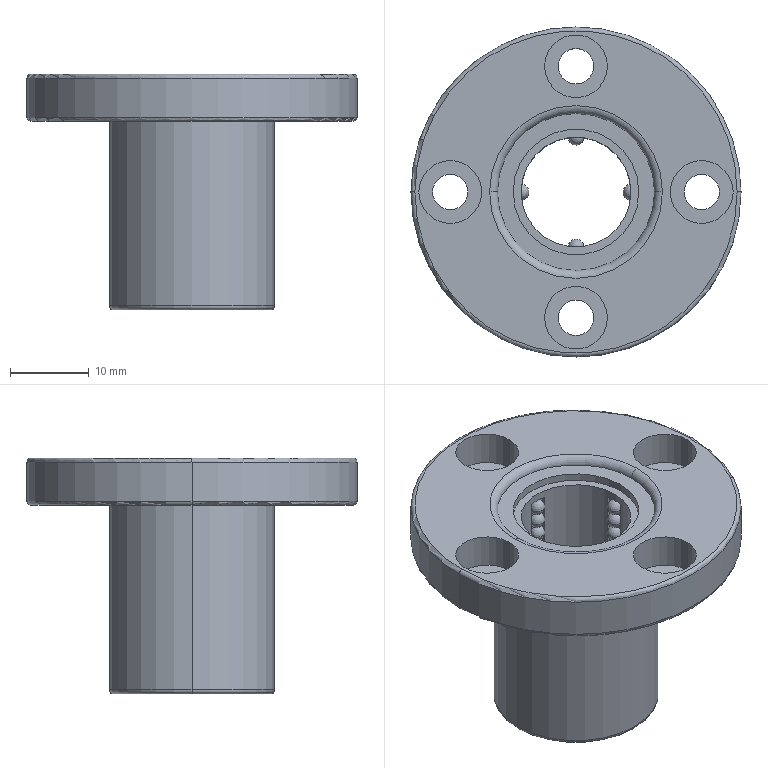Part | SolidWorks | features ICE 12, Fillet 2, Revolution 2, CirPattern 1, LPattern 1 | 1 solid | 157 faces | box 42 x 42 x 30 mm | volume 10856 mm3 | sphere 96 | plane 29 | cylinder 24 | torus 8 | commonest cylinder face diameters 4.5 x8 8 x8 13.99 x2 15.99 x2 21 x2 42 x2